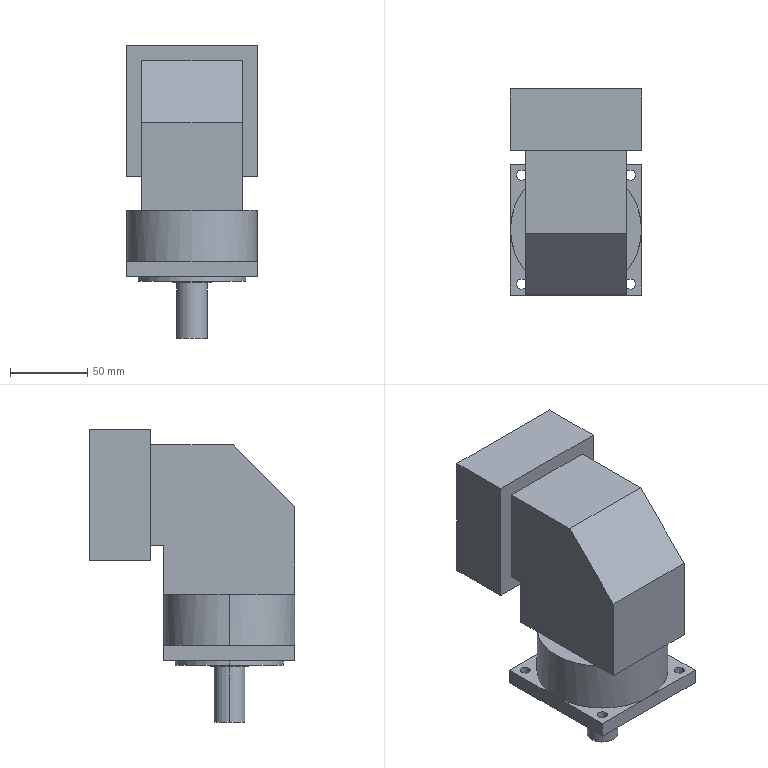Part | NX | features BREP 1 | 1 solid | 50 faces | box 85 x 133.5 x 190 mm | volume 1087253 mm3 | plane 32 | cylinder 18 | commonest cylinder face diameters 6.5 x8 20 x4 25 x2 70 x2 85 x2
STEP:
#1=CARTESIAN_POINT('',(32.5,27.386,83.2));
#2=VERTEX_POINT('',#1);
#3=CARTESIAN_POINT('',(42.5,0.,83.2));
#4=VERTEX_POINT('',#3);
#5=CARTESIAN_POINT('',(0.,0.,83.2));
#6=DIRECTION('',(0.,0.,-1.));
#7=DIRECTION('',(-1.,0.,0.));
#8=AXIS2_PLACEMENT_3D('',#5,#6,#7);
#9=CIRCLE('',#8,42.5);
#10=EDGE_CURVE('',#2,#4,#9,.T.);
#11=ORIENTED_EDGE('',*,*,#10,.T.);
#12=CARTESIAN_POINT('',(42.5,0.,50.));
#13=VERTEX_POINT('',#12);
#14=CARTESIAN_POINT('',(42.5,0.,83.2));
#15=DIRECTION('',(0.,0.,-1.));
#16=VECTOR('',#15,1000.);
#17=LINE('',#14,#16);
#18=EDGE_CURVE('',#4,#13,#17,.T.);
#19=ORIENTED_EDGE('',*,*,#18,.T.);
#20=CARTESIAN_POINT('',(0.,42.5,50.));
#21=VERTEX_POINT('',#20);
#22=CARTESIAN_POINT('',(0.,0.,50.));
#23=DIRECTION('',(0.,0.,1.));
#24=DIRECTION('',(-1.,0.,0.));
#25=AXIS2_PLACEMENT_3D('',#22,#23,#24);
#26=CIRCLE('',#25,42.5);
#27=EDGE_CURVE('',#13,#21,#26,.T.);
#28=ORIENTED_EDGE('',*,*,#27,.T.);
#29=CARTESIAN_POINT('',(-42.5,0.,50.));
#30=VERTEX_POINT('',#29);
#31=CARTESIAN_POINT('',(0.,0.,50.));
#32=DIRECTION('',(0.,0.,1.));
#33=DIRECTION('',(-1.,0.,0.));
#34=AXIS2_PLACEMENT_3D('',#31,#32,#33);
#35=CIRCLE('',#34,42.5);
#36=EDGE_CURVE('',#21,#30,#35,.T.);
#37=ORIENTED_EDGE('',*,*,#36,.T.);
#38=CARTESIAN_POINT('',(-42.5,0.,83.2));
#39=VERTEX_POINT('',#38);
#40=CARTESIAN_POINT('',(-42.5,0.,83.2));
#41=DIRECTION('',(0.,0.,-1.));
#42=VECTOR('',#41,1000.);
#43=LINE('',#40,#42);
#44=EDGE_CURVE('',#39,#30,#43,.T.);
#45=ORIENTED_EDGE('',*,*,#44,.F.);
#46=CARTESIAN_POINT('',(-32.5,27.386,83.2));
#47=VERTEX_POINT('',#46);
#48=CARTESIAN_POINT('',(0.,0.,83.2));
#49=DIRECTION('',(0.,0.,1.));
#50=DIRECTION('',(-1.,0.,0.));
#51=AXIS2_PLACEMENT_3D('',#48,#49,#50);
#52=CIRCLE('',#51,42.5);
#53=EDGE_CURVE('',#47,#39,#52,.T.);
#54=ORIENTED_EDGE('',*,*,#53,.F.);
#55=CARTESIAN_POINT('',(0.,42.5,83.2));
#56=VERTEX_POINT('',#55);
#57=CARTESIAN_POINT('',(0.,0.,83.2));
#58=DIRECTION('',(0.,0.,-1.));
#59=DIRECTION('',(-1.,0.,0.));
#60=AXIS2_PLACEMENT_3D('',#57,#58,#59);
#61=CIRCLE('',#60,42.5);
#62=EDGE_CURVE('',#47,#56,#61,.T.);
#63=ORIENTED_EDGE('',*,*,#62,.T.);
#64=CARTESIAN_POINT('',(0.,0.,83.2));
#65=DIRECTION('',(0.,0.,-1.));
#66=DIRECTION('',(-1.,0.,0.));
#67=AXIS2_PLACEMENT_3D('',#64,#65,#66);
#68=CIRCLE('',#67,42.5);
#69=EDGE_CURVE('',#56,#2,#68,.T.);
#70=ORIENTED_EDGE('',*,*,#69,.T.);
#71=EDGE_LOOP('',(#11,#19,#28,#37,#45,#54,#63,#70));
#72=FACE_BOUND('',#71,.T.);
#73=CARTESIAN_POINT('',(0.,0.,83.2));
#74=DIRECTION('',(0.,0.,-1.));
#75=DIRECTION('',(-1.,0.,0.));
#76=AXIS2_PLACEMENT_3D('',#73,#74,#75);
#77=CYLINDRICAL_SURFACE('',#76,42.5);
#78=ADVANCED_FACE('',(#72),#77,.T.);
#79=CARTESIAN_POINT('',(32.105,-35.355,50.));
#80=VERTEX_POINT('',#79);
#81=CARTESIAN_POINT('',(38.605,-35.355,50.));
#82=VERTEX_POINT('',#81);
#83=CARTESIAN_POINT('',(35.355,-35.355,50.));
#84=DIRECTION('',(0.,0.,1.));
#85=DIRECTION('',(-1.,0.,0.));
#86=AXIS2_PLACEMENT_3D('',#83,#84,#85);
#87=CIRCLE('',#86,3.25);
#88=EDGE_CURVE('',#80,#82,#87,.T.);
#89=ORIENTED_EDGE('',*,*,#88,.T.);
#90=CARTESIAN_POINT('',(38.605,-35.355,40.));
#91=VERTEX_POINT('',#90);
#92=CARTESIAN_POINT('',(38.605,-35.355,40.));
#93=DIRECTION('',(0.,0.,-1.));
#94=VECTOR('',#93,1000.);
#95=LINE('',#92,#94);
#96=EDGE_CURVE('',#82,#91,#95,.T.);
#97=ORIENTED_EDGE('',*,*,#96,.T.);
#98=CARTESIAN_POINT('',(32.105,-35.355,40.));
#99=VERTEX_POINT('',#98);
#100=CARTESIAN_POINT('',(35.355,-35.355,40.));
#101=DIRECTION('',(0.,0.,1.));
#102=DIRECTION('',(-1.,0.,0.));
#103=AXIS2_PLACEMENT_3D('',#100,#101,#102);
#104=CIRCLE('',#103,3.25);
#105=EDGE_CURVE('',#99,#91,#104,.T.);
#106=ORIENTED_EDGE('',*,*,#105,.F.);
#107=CARTESIAN_POINT('',(32.105,-35.355,40.));
#108=DIRECTION('',(0.,0.,-1.));
#109=VECTOR('',#108,1000.);
#110=LINE('',#107,#109);
#111=EDGE_CURVE('',#80,#99,#110,.T.);
#112=ORIENTED_EDGE('',*,*,#111,.F.);
#113=EDGE_LOOP('',(#89,#97,#106,#112));
#114=FACE_BOUND('',#113,.T.);
#115=CARTESIAN_POINT('',(35.355,-35.355,40.));
#116=DIRECTION('',(0.,0.,-1.));
#117=DIRECTION('',(-1.,0.,0.));
#118=AXIS2_PLACEMENT_3D('',#115,#116,#117);
#119=CYLINDRICAL_SURFACE('',#118,3.25);
#120=ADVANCED_FACE('',(#114),#119,.F.);
#121=CARTESIAN_POINT('',(-38.605,-35.355,50.));
#122=VERTEX_POINT('',#121);
#123=CARTESIAN_POINT('',(-32.105,-35.355,50.));
#124=VERTEX_POINT('',#123);
#125=CARTESIAN_POINT('',(-35.355,-35.355,50.));
#126=DIRECTION('',(0.,0.,1.));
#127=DIRECTION('',(-1.,0.,0.));
#128=AXIS2_PLACEMENT_3D('',#125,#126,#127);
#129=CIRCLE('',#128,3.25);
#130=EDGE_CURVE('',#122,#124,#129,.T.);
#131=ORIENTED_EDGE('',*,*,#130,.T.);
#132=CARTESIAN_POINT('',(-32.105,-35.355,40.));
#133=VERTEX_POINT('',#132);
#134=CARTESIAN_POINT('',(-32.105,-35.355,40.));
#135=DIRECTION('',(0.,0.,-1.));
#136=VECTOR('',#135,1000.);
#137=LINE('',#134,#136);
#138=EDGE_CURVE('',#124,#133,#137,.T.);
#139=ORIENTED_EDGE('',*,*,#138,.T.);
#140=CARTESIAN_POINT('',(-38.605,-35.355,40.));
#141=VERTEX_POINT('',#140);
#142=CARTESIAN_POINT('',(-35.355,-35.355,40.));
#143=DIRECTION('',(0.,0.,1.));
#144=DIRECTION('',(-1.,0.,0.));
#145=AXIS2_PLACEMENT_3D('',#142,#143,#144);
#146=CIRCLE('',#145,3.25);
#147=EDGE_CURVE('',#141,#133,#146,.T.);
#148=ORIENTED_EDGE('',*,*,#147,.F.);
#149=CARTESIAN_POINT('',(-38.605,-35.355,40.));
#150=DIRECTION('',(0.,0.,-1.));
#151=VECTOR('',#150,1000.);
#152=LINE('',#149,#151);
#153=EDGE_CURVE('',#122,#141,#152,.T.);
#154=ORIENTED_EDGE('',*,*,#153,.F.);
#155=EDGE_LOOP('',(#131,#139,#148,#154));
#156=FACE_BOUND('',#155,.T.);
#157=CARTESIAN_POINT('',(-35.355,-35.355,40.));
#158=DIRECTION('',(0.,0.,-1.));
#159=DIRECTION('',(-1.,0.,0.));
#160=AXIS2_PLACEMENT_3D('',#157,#158,#159);
#161=CYLINDRICAL_SURFACE('',#160,3.25);
#162=ADVANCED_FACE('',(#156),#161,.F.);
#163=CARTESIAN_POINT('',(-38.605,35.355,50.));
#164=VERTEX_POINT('',#163);
#165=CARTESIAN_POINT('',(-32.105,35.355,50.));
#166=VERTEX_POINT('',#165);
#167=CARTESIAN_POINT('',(-35.355,35.355,50.));
#168=DIRECTION('',(0.,0.,1.));
#169=DIRECTION('',(-1.,0.,0.));
#170=AXIS2_PLACEMENT_3D('',#167,#168,#169);
#171=CIRCLE('',#170,3.25);
#172=EDGE_CURVE('',#164,#166,#171,.T.);
#173=ORIENTED_EDGE('',*,*,#172,.T.);
#174=CARTESIAN_POINT('',(-32.105,35.355,40.));
#175=VERTEX_POINT('',#174);
#176=CARTESIAN_POINT('',(-32.105,35.355,40.));
#177=DIRECTION('',(0.,0.,-1.));
#178=VECTOR('',#177,1000.);
#179=LINE('',#176,#178);
#180=EDGE_CURVE('',#166,#175,#179,.T.);
#181=ORIENTED_EDGE('',*,*,#180,.T.);
#182=CARTESIAN_POINT('',(-38.605,35.355,40.));
#183=VERTEX_POINT('',#182);
#184=CARTESIAN_POINT('',(-35.355,35.355,40.));
#185=DIRECTION('',(0.,0.,1.));
#186=DIRECTION('',(-1.,0.,0.));
#187=AXIS2_PLACEMENT_3D('',#184,#185,#186);
#188=CIRCLE('',#187,3.25);
#189=EDGE_CURVE('',#183,#175,#188,.T.);
#190=ORIENTED_EDGE('',*,*,#189,.F.);
#191=CARTESIAN_POINT('',(-38.605,35.355,40.));
#192=DIRECTION('',(0.,0.,-1.));
#193=VECTOR('',#192,1000.);
#194=LINE('',#191,#193);
#195=EDGE_CURVE('',#164,#183,#194,.T.);
#196=ORIENTED_EDGE('',*,*,#195,.F.);
#197=EDGE_LOOP('',(#173,#181,#190,#196));
#198=FACE_BOUND('',#197,.T.);
#199=CARTESIAN_POINT('',(-35.355,35.355,40.));
#200=DIRECTION('',(0.,0.,-1.));
#201=DIRECTION('',(-1.,0.,0.));
#202=AXIS2_PLACEMENT_3D('',#199,#200,#201);
#203=CYLINDRICAL_SURFACE('',#202,3.25);
#204=ADVANCED_FACE('',(#198),#203,.F.);
#205=CARTESIAN_POINT('',(32.105,35.355,50.));
#206=VERTEX_POINT('',#205);
#207=CARTESIAN_POINT('',(38.605,35.355,50.));
#208=VERTEX_POINT('',#207);
#209=CARTESIAN_POINT('',(35.355,35.355,50.));
#210=DIRECTION('',(0.,0.,1.));
#211=DIRECTION('',(-1.,0.,0.));
#212=AXIS2_PLACEMENT_3D('',#209,#210,#211);
#213=CIRCLE('',#212,3.25);
#214=EDGE_CURVE('',#206,#208,#213,.T.);
#215=ORIENTED_EDGE('',*,*,#214,.T.);
#216=CARTESIAN_POINT('',(38.605,35.355,40.));
#217=VERTEX_POINT('',#216);
#218=CARTESIAN_POINT('',(38.605,35.355,40.));
#219=DIRECTION('',(0.,0.,-1.));
#220=VECTOR('',#219,1000.);
#221=LINE('',#218,#220);
#222=EDGE_CURVE('',#208,#217,#221,.T.);
#223=ORIENTED_EDGE('',*,*,#222,.T.);
#224=CARTESIAN_POINT('',(32.105,35.355,40.));
#225=VERTEX_POINT('',#224);
#226=CARTESIAN_POINT('',(35.355,35.355,40.));
#227=DIRECTION('',(0.,0.,1.));
#228=DIRECTION('',(-1.,0.,0.));
#229=AXIS2_PLACEMENT_3D('',#226,#227,#228);
#230=CIRCLE('',#229,3.25);
#231=EDGE_CURVE('',#225,#217,#230,.T.);
#232=ORIENTED_EDGE('',*,*,#231,.F.);
#233=CARTESIAN_POINT('',(32.105,35.355,40.));
#234=DIRECTION('',(0.,0.,-1.));
#235=VECTOR('',#234,1000.);
#236=LINE('',#233,#235);
#237=EDGE_CURVE('',#206,#225,#236,.T.);
#238=ORIENTED_EDGE('',*,*,#237,.F.);
#239=EDGE_LOOP('',(#215,#223,#232,#238));
#240=FACE_BOUND('',#239,.T.);
#241=CARTESIAN_POINT('',(35.355,35.355,40.));
#242=DIRECTION('',(0.,0.,-1.));
#243=DIRECTION('',(-1.,0.,0.));
#244=AXIS2_PLACEMENT_3D('',#241,#242,#243);
#245=CYLINDRICAL_SURFACE('',#244,3.25);
#246=ADVANCED_FACE('',(#240),#245,.F.);
#247=CARTESIAN_POINT('',(0.,81.,137.5));
#248=VERTEX_POINT('',#247);
#249=CARTESIAN_POINT('',(0.,81.,157.5));
#250=VERTEX_POINT('',#249);
#251=CARTESIAN_POINT('',(0.,81.,147.5));
#252=DIRECTION('',(0.,1.,0.));
#253=DIRECTION('',(0.,0.,1.));
#254=AXIS2_PLACEMENT_3D('',#251,#252,#253);
#255=CIRCLE('',#254,10.);
#256=EDGE_CURVE('',#248,#250,#255,.T.);
#257=ORIENTED_EDGE('',*,*,#256,.F.);
#258=CARTESIAN_POINT('',(0.,91.,137.5));
#259=VERTEX_POINT('',#258);
#260=CARTESIAN_POINT('',(0.,81.,137.5));
#261=DIRECTION('',(0.,1.,0.));
#262=VECTOR('',#261,1000.);
#263=LINE('',#260,#262);
#264=EDGE_CURVE('',#259,#248,#263,.F.);
#265=ORIENTED_EDGE('',*,*,#264,.F.);
#266=CARTESIAN_POINT('',(0.,91.,157.5));
#267=VERTEX_POINT('',#266);
#268=CARTESIAN_POINT('',(0.,91.,147.5));
#269=DIRECTION('',(0.,1.,0.));
#270=DIRECTION('',(0.,0.,1.));
#271=AXIS2_PLACEMENT_3D('',#268,#269,#270);
#272=CIRCLE('',#271,10.);
#273=EDGE_CURVE('',#259,#267,#272,.T.);
#274=ORIENTED_EDGE('',*,*,#273,.T.);
#275=CARTESIAN_POINT('',(0.,81.,157.5));
#276=DIRECTION('',(0.,1.,0.));
#277=VECTOR('',#276,1000.);
#278=LINE('',#275,#277);
#279=EDGE_CURVE('',#267,#250,#278,.F.);
#280=ORIENTED_EDGE('',*,*,#279,.T.);
#281=EDGE_LOOP('',(#257,#265,#274,#280));
#282=FACE_BOUND('',#281,.T.);
#283=CARTESIAN_POINT('',(0.,81.,147.5));
#284=DIRECTION('',(0.,1.,0.));
#285=DIRECTION('',(0.,0.,1.));
#286=AXIS2_PLACEMENT_3D('',#283,#284,#285);
#287=CYLINDRICAL_SURFACE('',#286,10.);
#288=ADVANCED_FACE('',(#282),#287,.F.);
#289=CARTESIAN_POINT('',(-35.,0.,40.));
#290=VERTEX_POINT('',#289);
#291=CARTESIAN_POINT('',(35.,0.,40.));
#292=VERTEX_POINT('',#291);
#293=CARTESIAN_POINT('',(0.,0.,40.));
#294=DIRECTION('',(0.,0.,-1.));
#295=DIRECTION('',(-1.,0.,0.));
#296=AXIS2_PLACEMENT_3D('',#293,#294,#295);
#297=CIRCLE('',#296,35.);
#298=EDGE_CURVE('',#290,#292,#297,.T.);
#299=ORIENTED_EDGE('',*,*,#298,.T.);
#300=CARTESIAN_POINT('',(35.,0.,37.));
#301=VERTEX_POINT('',#300);
#302=CARTESIAN_POINT('',(35.,0.,40.));
#303=DIRECTION('',(0.,0.,-1.));
#304=VECTOR('',#303,1000.);
#305=LINE('',#302,#304);
#306=EDGE_CURVE('',#292,#301,#305,.T.);
#307=ORIENTED_EDGE('',*,*,#306,.T.);
#308=CARTESIAN_POINT('',(-35.,0.,37.));
#309=VERTEX_POINT('',#308);
#310=CARTESIAN_POINT('',(0.,0.,37.));
#311=DIRECTION('',(0.,0.,1.));
#312=DIRECTION('',(-1.,0.,0.));
#313=AXIS2_PLACEMENT_3D('',#310,#311,#312);
#314=CIRCLE('',#313,35.);
#315=EDGE_CURVE('',#301,#309,#314,.T.);
#316=ORIENTED_EDGE('',*,*,#315,.T.);
#317=CARTESIAN_POINT('',(-35.,0.,40.));
#318=DIRECTION('',(0.,0.,-1.));
#319=VECTOR('',#318,1000.);
#320=LINE('',#317,#319);
#321=EDGE_CURVE('',#290,#309,#320,.T.);
#322=ORIENTED_EDGE('',*,*,#321,.F.);
#323=EDGE_LOOP('',(#299,#307,#316,#322));
#324=FACE_BOUND('',#323,.T.);
#325=CARTESIAN_POINT('',(0.,0.,40.));
#326=DIRECTION('',(0.,0.,-1.));
#327=DIRECTION('',(-1.,0.,0.));
#328=AXIS2_PLACEMENT_3D('',#325,#326,#327);
#329=CYLINDRICAL_SURFACE('',#328,35.);
#330=ADVANCED_FACE('',(#324),#329,.T.);
#331=CARTESIAN_POINT('',(-12.5,0.,37.));
#332=VERTEX_POINT('',#331);
#333=CARTESIAN_POINT('',(12.5,0.,37.));
#334=VERTEX_POINT('',#333);
#335=CARTESIAN_POINT('',(0.,0.,37.));
#336=DIRECTION('',(0.,0.,-1.));
#337=DIRECTION('',(-1.,0.,0.));
#338=AXIS2_PLACEMENT_3D('',#335,#336,#337);
#339=CIRCLE('',#338,12.5);
#340=EDGE_CURVE('',#332,#334,#339,.T.);
#341=ORIENTED_EDGE('',*,*,#340,.T.);
#342=CARTESIAN_POINT('',(12.5,0.,36.));
#343=VERTEX_POINT('',#342);
#344=CARTESIAN_POINT('',(12.5,0.,37.));
#345=DIRECTION('',(0.,0.,-1.));
#346=VECTOR('',#345,1000.);
#347=LINE('',#344,#346);
#348=EDGE_CURVE('',#334,#343,#347,.T.);
#349=ORIENTED_EDGE('',*,*,#348,.T.);
#350=CARTESIAN_POINT('',(-12.5,0.,36.));
#351=VERTEX_POINT('',#350);
#352=CARTESIAN_POINT('',(0.,0.,36.));
#353=DIRECTION('',(0.,0.,1.));
#354=DIRECTION('',(-1.,0.,0.));
#355=AXIS2_PLACEMENT_3D('',#352,#353,#354);
#356=CIRCLE('',#355,12.5);
#357=EDGE_CURVE('',#343,#351,#356,.T.);
#358=ORIENTED_EDGE('',*,*,#357,.T.);
#359=CARTESIAN_POINT('',(-12.5,0.,37.));
#360=DIRECTION('',(0.,0.,-1.));
#361=VECTOR('',#360,1000.);
#362=LINE('',#359,#361);
#363=EDGE_CURVE('',#332,#351,#362,.T.);
#364=ORIENTED_EDGE('',*,*,#363,.F.);
#365=EDGE_LOOP('',(#341,#349,#358,#364));
#366=FACE_BOUND('',#365,.T.);
#367=CARTESIAN_POINT('',(0.,0.,37.));
#368=DIRECTION('',(0.,0.,-1.));
#369=DIRECTION('',(-1.,0.,0.));
#370=AXIS2_PLACEMENT_3D('',#367,#368,#369);
#371=CYLINDRICAL_SURFACE('',#370,12.5);
#372=ADVANCED_FACE('',(#366),#371,.T.);
#373=CARTESIAN_POINT('',(-10.,0.,36.));
#374=VERTEX_POINT('',#373);
#375=CARTESIAN_POINT('',(10.,0.,36.));
#376=VERTEX_POINT('',#375);
#377=CARTESIAN_POINT('',(0.,0.,36.));
#378=DIRECTION('',(0.,0.,-1.));
#379=DIRECTION('',(-1.,0.,0.));
#380=AXIS2_PLACEMENT_3D('',#377,#378,#379);
#381=CIRCLE('',#380,10.);
#382=EDGE_CURVE('',#374,#376,#381,.T.);
#383=ORIENTED_EDGE('',*,*,#382,.T.);
#384=CARTESIAN_POINT('',(10.,0.,0.));
#385=VERTEX_POINT('',#384);
#386=CARTESIAN_POINT('',(10.,0.,36.));
#387=DIRECTION('',(0.,0.,-1.));
#388=VECTOR('',#387,1000.);
#389=LINE('',#386,#388);
#390=EDGE_CURVE('',#376,#385,#389,.T.);
#391=ORIENTED_EDGE('',*,*,#390,.T.);
#392=CARTESIAN_POINT('',(-10.,0.,0.));
#393=VERTEX_POINT('',#392);
#394=CARTESIAN_POINT('',(0.,0.,0.));
#395=DIRECTION('',(0.,0.,1.));
#396=DIRECTION('',(-1.,0.,0.));
#397=AXIS2_PLACEMENT_3D('',#394,#395,#396);
#398=CIRCLE('',#397,10.);
#399=EDGE_CURVE('',#385,#393,#398,.T.);
#400=ORIENTED_EDGE('',*,*,#399,.T.);
#401=CARTESIAN_POINT('',(-10.,0.,36.));
#402=DIRECTION('',(0.,0.,-1.));
#403=VECTOR('',#402,1000.);
#404=LINE('',#401,#403);
#405=EDGE_CURVE('',#374,#393,#404,.T.);
#406=ORIENTED_EDGE('',*,*,#405,.F.);
#407=EDGE_LOOP('',(#383,#391,#400,#406));
#408=FACE_BOUND('',#407,.T.);
#409=CARTESIAN_POINT('',(0.,0.,36.));
#410=DIRECTION('',(0.,0.,-1.));
#411=DIRECTION('',(-1.,0.,0.));
#412=AXIS2_PLACEMENT_3D('',#409,#410,#411);
#413=CYLINDRICAL_SURFACE('',#412,10.);
#414=ADVANCED_FACE('',(#408),#413,.T.);
#415=CARTESIAN_POINT('',(-32.5,-42.5,83.2));
#416=VERTEX_POINT('',#415);
#417=CARTESIAN_POINT('',(-32.5,-42.5,140.));
#418=VERTEX_POINT('',#417);
#419=CARTESIAN_POINT('',(-32.5,-42.5,180.));
#420=DIRECTION('',(0.,0.,1.));
#421=VECTOR('',#420,1000.);
#422=LINE('',#419,#421);
#423=EDGE_CURVE('',#416,#418,#422,.T.);
#424=ORIENTED_EDGE('',*,*,#423,.T.);
#425=CARTESIAN_POINT('',(-32.5,-2.5,180.));
#426=VERTEX_POINT('',#425);
#427=CARTESIAN_POINT('',(-32.5,-42.5,140.));
#428=DIRECTION('',(0.,0.7071,0.7071));
#429=VECTOR('',#428,1000.);
#430=LINE('',#427,#429);
#431=EDGE_CURVE('',#418,#426,#430,.T.);
#432=ORIENTED_EDGE('',*,*,#431,.T.);
#433=CARTESIAN_POINT('',(-32.5,51.,180.));
#434=VERTEX_POINT('',#433);
#435=CARTESIAN_POINT('',(-32.5,-42.5,180.));
#436=DIRECTION('',(0.,1.,0.));
#437=VECTOR('',#436,1000.);
#438=LINE('',#435,#437);
#439=EDGE_CURVE('',#426,#434,#438,.T.);
#440=ORIENTED_EDGE('',*,*,#439,.T.);
#441=CARTESIAN_POINT('',(-32.5,51.,115.));
#442=VERTEX_POINT('',#441);
#443=CARTESIAN_POINT('',(-32.5,51.,180.));
#444=DIRECTION('',(0.,0.,-1.));
#445=VECTOR('',#444,1000.);
#446=LINE('',#443,#445);
#447=EDGE_CURVE('',#434,#442,#446,.T.);
#448=ORIENTED_EDGE('',*,*,#447,.T.);
#449=CARTESIAN_POINT('',(-32.5,42.5,115.));
#450=VERTEX_POINT('',#449);
#451=CARTESIAN_POINT('',(-32.5,-42.5,115.));
#452=DIRECTION('',(0.,-1.,0.));
#453=VECTOR('',#452,1000.);
#454=LINE('',#451,#453);
#455=EDGE_CURVE('',#442,#450,#454,.T.);
#456=ORIENTED_EDGE('',*,*,#455,.T.);
#457=CARTESIAN_POINT('',(-32.5,42.5,83.2));
#458=VERTEX_POINT('',#457);
#459=CARTESIAN_POINT('',(-32.5,42.5,180.));
#460=DIRECTION('',(0.,0.,-1.));
#461=VECTOR('',#460,1000.);
#462=LINE('',#459,#461);
#463=EDGE_CURVE('',#450,#458,#462,.T.);
#464=ORIENTED_EDGE('',*,*,#463,.T.);
#465=CARTESIAN_POINT('',(-32.5,-42.5,83.2));
#466=DIRECTION('',(0.,-1.,0.));
#467=VECTOR('',#466,1000.);
#468=LINE('',#465,#467);
#469=EDGE_CURVE('',#458,#47,#468,.T.);
#470=ORIENTED_EDGE('',*,*,#469,.T.);
#471=CARTESIAN_POINT('',(-32.5,-27.386,83.2));
#472=VERTEX_POINT('',#471);
#473=CARTESIAN_POINT('',(-32.5,-42.5,83.2));
#474=DIRECTION('',(0.,-1.,0.));
#475=VECTOR('',#474,1000.);
#476=LINE('',#473,#475);
#477=EDGE_CURVE('',#47,#472,#476,.T.);
#478=ORIENTED_EDGE('',*,*,#477,.T.);
#479=CARTESIAN_POINT('',(-32.5,-42.5,83.2));
#480=DIRECTION('',(0.,-1.,0.));
#481=VECTOR('',#480,1000.);
#482=LINE('',#479,#481);
#483=EDGE_CURVE('',#472,#416,#482,.T.);
#484=ORIENTED_EDGE('',*,*,#483,.T.);
#485=EDGE_LOOP('',(#424,#432,#440,#448,#456,#464,#470,#478,#484));
#486=FACE_BOUND('',#485,.T.);
#487=CARTESIAN_POINT('',(-32.5,-42.5,180.));
#488=DIRECTION('',(-1.,0.,0.));
#489=DIRECTION('',(0.,0.,1.));
#490=AXIS2_PLACEMENT_3D('',#487,#488,#489);
#491=PLANE('',#490);
#492=ADVANCED_FACE('',(#486),#491,.T.);
#493=CARTESIAN_POINT('',(32.5,-42.5,140.));
#494=VERTEX_POINT('',#493);
#495=CARTESIAN_POINT('',(32.5,-42.5,140.));
#496=DIRECTION('',(-1.,0.,0.));
#497=VECTOR('',#496,1000.);
#498=LINE('',#495,#497);
#499=EDGE_CURVE('',#494,#418,#498,.T.);
#500=ORIENTED_EDGE('',*,*,#499,.F.);
#501=CARTESIAN_POINT('',(32.5,-2.5,180.));
#502=VERTEX_POINT('',#501);
#503=CARTESIAN_POINT('',(32.5,-2.5,180.));
#504=DIRECTION('',(0.,-0.7071,-0.7071));
#505=VECTOR('',#504,1000.);
#506=LINE('',#503,#505);
#507=EDGE_CURVE('',#502,#494,#506,.T.);
#508=ORIENTED_EDGE('',*,*,#507,.F.);
#509=CARTESIAN_POINT('',(32.5,-2.5,180.));
#510=DIRECTION('',(1.,0.,0.));
#511=VECTOR('',#510,1000.);
#512=LINE('',#509,#511);
#513=EDGE_CURVE('',#426,#502,#512,.T.);
#514=ORIENTED_EDGE('',*,*,#513,.F.);
#515=ORIENTED_EDGE('',*,*,#431,.F.);
#516=EDGE_LOOP('',(#500,#508,#514,#515));
#517=FACE_BOUND('',#516,.T.);
#518=CARTESIAN_POINT('',(32.5,-2.5,180.));
#519=DIRECTION('',(0.,0.7071,-0.7071));
#520=DIRECTION('',(-1.,0.,0.));
#521=AXIS2_PLACEMENT_3D('',#518,#519,#520);
#522=PLANE('',#521);
#523=ADVANCED_FACE('',(#517),#522,.F.);
#524=CARTESIAN_POINT('',(0.,-42.5,83.2));
#525=VERTEX_POINT('',#524);
#526=CARTESIAN_POINT('',(32.5,-42.5,83.2));
#527=DIRECTION('',(-1.,0.,0.));
#528=VECTOR('',#527,1000.);
#529=LINE('',#526,#528);
#530=EDGE_CURVE('',#525,#416,#529,.T.);
#531=ORIENTED_EDGE('',*,*,#530,.F.);
#532=CARTESIAN_POINT('',(32.5,-42.5,83.2));
#533=VERTEX_POINT('',#532);
#534=CARTESIAN_POINT('',(32.5,-42.5,83.2));
#535=DIRECTION('',(-1.,0.,0.));
#536=VECTOR('',#535,1000.);
#537=LINE('',#534,#536);
#538=EDGE_CURVE('',#533,#525,#537,.T.);
#539=ORIENTED_EDGE('',*,*,#538,.F.);
#540=CARTESIAN_POINT('',(32.5,-42.5,83.2));
#541=DIRECTION('',(0.,0.,-1.));
#542=VECTOR('',#541,1000.);
#543=LINE('',#540,#542);
#544=EDGE_CURVE('',#494,#533,#543,.T.);
#545=ORIENTED_EDGE('',*,*,#544,.F.);
#546=ORIENTED_EDGE('',*,*,#499,.T.);
#547=ORIENTED_EDGE('',*,*,#423,.F.);
#548=EDGE_LOOP('',(#531,#539,#545,#546,#547));
#549=FACE_BOUND('',#548,.T.);
#550=CARTESIAN_POINT('',(32.5,-42.5,83.2));
#551=DIRECTION('',(0.,1.,0.));
#552=DIRECTION('',(0.,0.,-1.));
#553=AXIS2_PLACEMENT_3D('',#550,#551,#552);
#554=PLANE('',#553);
#555=ADVANCED_FACE('',(#549),#554,.F.);
#556=CARTESIAN_POINT('',(0.,0.,83.2));
#557=DIRECTION('',(0.,0.,-1.));
#558=DIRECTION('',(-1.,0.,0.));
#559=AXIS2_PLACEMENT_3D('',#556,#557,#558);
#560=CIRCLE('',#559,42.5);
#561=EDGE_CURVE('',#525,#472,#560,.T.);
#562=ORIENTED_EDGE('',*,*,#561,.F.);
#563=ORIENTED_EDGE('',*,*,#530,.T.);
#564=ORIENTED_EDGE('',*,*,#483,.F.);
#565=EDGE_LOOP('',(#562,#563,#564));
#566=FACE_BOUND('',#565,.T.);
#567=CARTESIAN_POINT('',(32.5,42.5,83.2));
#568=DIRECTION('',(0.,0.,1.));
#569=DIRECTION('',(1.,0.,0.));
#570=AXIS2_PLACEMENT_3D('',#567,#568,#569);
#571=PLANE('',#570);
#572=ADVANCED_FACE('',(#566),#571,.F.);
#573=ORIENTED_EDGE('',*,*,#53,.T.);
#574=CARTESIAN_POINT('',(0.,0.,83.2));
#575=DIRECTION('',(0.,0.,1.));
#576=DIRECTION('',(-1.,0.,0.));
#577=AXIS2_PLACEMENT_3D('',#574,#575,#576);
#578=CIRCLE('',#577,42.5);
#579=EDGE_CURVE('',#39,#472,#578,.T.);
#580=ORIENTED_EDGE('',*,*,#579,.T.);
#581=ORIENTED_EDGE('',*,*,#477,.F.);
#582=EDGE_LOOP('',(#573,#580,#581));
#583=FACE_BOUND('',#582,.T.);
#584=CARTESIAN_POINT('',(-42.5,42.5,83.2));
#585=DIRECTION('',(0.,0.,1.));
#586=DIRECTION('',(1.,0.,0.));
#587=AXIS2_PLACEMENT_3D('',#584,#585,#586);
#588=PLANE('',#587);
#589=ADVANCED_FACE('',(#583),#588,.T.);
#590=ORIENTED_EDGE('',*,*,#62,.F.);
#591=ORIENTED_EDGE('',*,*,#469,.F.);
#592=CARTESIAN_POINT('',(32.5,42.5,83.2));
#593=DIRECTION('',(-1.,0.,0.));
#594=VECTOR('',#593,1000.);
#595=LINE('',#592,#594);
#596=EDGE_CURVE('',#56,#458,#595,.T.);
#597=ORIENTED_EDGE('',*,*,#596,.F.);
#598=EDGE_LOOP('',(#590,#591,#597));
#599=FACE_BOUND('',#598,.T.);
#600=CARTESIAN_POINT('',(32.5,42.5,83.2));
#601=DIRECTION('',(0.,0.,1.));
#602=DIRECTION('',(1.,0.,0.));
#603=AXIS2_PLACEMENT_3D('',#600,#601,#602);
#604=PLANE('',#603);
#605=ADVANCED_FACE('',(#599),#604,.F.);
#606=CARTESIAN_POINT('',(32.5,42.5,115.));
#607=VERTEX_POINT('',#606);
#608=CARTESIAN_POINT('',(32.5,42.5,115.));
#609=DIRECTION('',(-1.,0.,0.));
#610=VECTOR('',#609,1000.);
#611=LINE('',#608,#610);
#612=EDGE_CURVE('',#607,#450,#611,.T.);
#613=ORIENTED_EDGE('',*,*,#612,.F.);
#614=CARTESIAN_POINT('',(32.5,42.5,83.2));
#615=VERTEX_POINT('',#614);
#616=CARTESIAN_POINT('',(32.5,42.5,83.2));
#617=DIRECTION('',(0.,0.,1.));
#618=VECTOR('',#617,1000.);
#619=LINE('',#616,#618);
#620=EDGE_CURVE('',#615,#607,#619,.T.);
#621=ORIENTED_EDGE('',*,*,#620,.F.);
#622=CARTESIAN_POINT('',(32.5,42.5,83.2));
#623=DIRECTION('',(1.,0.,0.));
#624=VECTOR('',#623,1000.);
#625=LINE('',#622,#624);
#626=EDGE_CURVE('',#56,#615,#625,.T.);
#627=ORIENTED_EDGE('',*,*,#626,.F.);
#628=ORIENTED_EDGE('',*,*,#596,.T.);
#629=ORIENTED_EDGE('',*,*,#463,.F.);
#630=EDGE_LOOP('',(#613,#621,#627,#628,#629));
#631=FACE_BOUND('',#630,.T.);
#632=CARTESIAN_POINT('',(32.5,42.5,83.2));
#633=DIRECTION('',(0.,-1.,0.));
#634=DIRECTION('',(0.,0.,-1.));
#635=AXIS2_PLACEMENT_3D('',#632,#633,#634);
#636=PLANE('',#635);
#637=ADVANCED_FACE('',(#631),#636,.F.);
#638=CARTESIAN_POINT('',(32.5,51.,115.));
#639=VERTEX_POINT('',#638);
#640=CARTESIAN_POINT('',(32.5,51.,115.));
#641=DIRECTION('',(-1.,0.,0.));
#642=VECTOR('',#641,1000.);
#643=LINE('',#640,#642);
#644=EDGE_CURVE('',#639,#442,#643,.T.);
#645=ORIENTED_EDGE('',*,*,#644,.F.);
#646=CARTESIAN_POINT('',(32.5,42.5,115.));
#647=DIRECTION('',(0.,1.,0.));
#648=VECTOR('',#647,1000.);
#649=LINE('',#646,#648);
#650=EDGE_CURVE('',#607,#639,#649,.T.);
#651=ORIENTED_EDGE('',*,*,#650,.F.);
#652=ORIENTED_EDGE('',*,*,#612,.T.);
#653=ORIENTED_EDGE('',*,*,#455,.F.);
#654=EDGE_LOOP('',(#645,#651,#652,#653));
#655=FACE_BOUND('',#654,.T.);
#656=CARTESIAN_POINT('',(32.5,42.5,115.));
#657=DIRECTION('',(0.,0.,1.));
#658=DIRECTION('',(1.,0.,0.));
#659=AXIS2_PLACEMENT_3D('',#656,#657,#658);
#660=PLANE('',#659);
#661=ADVANCED_FACE('',(#655),#660,.F.);
#662=CARTESIAN_POINT('',(42.5,51.,105.));
#663=VERTEX_POINT('',#662);
#664=CARTESIAN_POINT('',(-42.5,51.,105.));
#665=VERTEX_POINT('',#664);
#666=CARTESIAN_POINT('',(42.5,51.,105.));
#667=DIRECTION('',(-1.,0.,0.));
#668=VECTOR('',#667,1000.);
#669=LINE('',#666,#668);
#670=EDGE_CURVE('',#663,#665,#669,.T.);
#671=ORIENTED_EDGE('',*,*,#670,.F.);
#672=CARTESIAN_POINT('',(42.5,51.,190.));
#673=VERTEX_POINT('',#672);
#674=CARTESIAN_POINT('',(42.5,51.,190.));
#675=DIRECTION('',(0.,0.,-1.));
#676=VECTOR('',#675,1000.);
#677=LINE('',#674,#676);
#678=EDGE_CURVE('',#673,#663,#677,.T.);
#679=ORIENTED_EDGE('',*,*,#678,.F.);
#680=CARTESIAN_POINT('',(-42.5,51.,190.));
#681=VERTEX_POINT('',#680);
#682=CARTESIAN_POINT('',(42.5,51.,190.));
#683=DIRECTION('',(1.,0.,0.));
#684=VECTOR('',#683,1000.);
#685=LINE('',#682,#684);
#686=EDGE_CURVE('',#681,#673,#685,.T.);
#687=ORIENTED_EDGE('',*,*,#686,.F.);
#688=CARTESIAN_POINT('',(-42.5,51.,190.));
#689=DIRECTION('',(0.,0.,1.));
#690=VECTOR('',#689,1000.);
#691=LINE('',#688,#690);
#692=EDGE_CURVE('',#665,#681,#691,.T.);
#693=ORIENTED_EDGE('',*,*,#692,.F.);
#694=EDGE_LOOP('',(#671,#679,#687,#693));
#695=FACE_BOUND('',#694,.T.);
#696=CARTESIAN_POINT('',(32.5,51.,180.));
#697=VERTEX_POINT('',#696);
#698=CARTESIAN_POINT('',(32.5,51.,190.));
#699=DIRECTION('',(0.,0.,1.));
#700=VECTOR('',#699,1000.);
#701=LINE('',#698,#700);
#702=EDGE_CURVE('',#639,#697,#701,.T.);
#703=ORIENTED_EDGE('',*,*,#702,.F.);
#704=ORIENTED_EDGE('',*,*,#644,.T.);
#705=ORIENTED_EDGE('',*,*,#447,.F.);
#706=CARTESIAN_POINT('',(42.5,51.,180.));
#707=DIRECTION('',(-1.,0.,0.));
#708=VECTOR('',#707,1000.);
#709=LINE('',#706,#708);
#710=EDGE_CURVE('',#697,#434,#709,.T.);
#711=ORIENTED_EDGE('',*,*,#710,.F.);
#712=EDGE_LOOP('',(#703,#704,#705,#711));
#713=FACE_BOUND('',#712,.T.);
#714=CARTESIAN_POINT('',(42.5,51.,190.));
#715=DIRECTION('',(0.,1.,0.));
#716=DIRECTION('',(1.,0.,0.));
#717=AXIS2_PLACEMENT_3D('',#714,#715,#716);
#718=PLANE('',#717);
#719=ADVANCED_FACE('',(#695,#713),#718,.F.);
#720=ORIENTED_EDGE('',*,*,#513,.T.);
#721=CARTESIAN_POINT('',(32.5,51.,180.));
#722=DIRECTION('',(0.,-1.,0.));
#723=VECTOR('',#722,1000.);
#724=LINE('',#721,#723);
#725=EDGE_CURVE('',#697,#502,#724,.T.);
#726=ORIENTED_EDGE('',*,*,#725,.F.);
#727=ORIENTED_EDGE('',*,*,#710,.T.);
#728=ORIENTED_EDGE('',*,*,#439,.F.);
#729=EDGE_LOOP('',(#720,#726,#727,#728));
#730=FACE_BOUND('',#729,.T.);
#731=CARTESIAN_POINT('',(32.5,51.,180.));
#732=DIRECTION('',(0.,0.,-1.));
#733=DIRECTION('',(0.,-1.,0.));
#734=AXIS2_PLACEMENT_3D('',#731,#732,#733);
#735=PLANE('',#734);
#736=ADVANCED_FACE('',(#730),#735,.F.);
#737=ORIENTED_EDGE('',*,*,#507,.T.);
#738=ORIENTED_EDGE('',*,*,#544,.T.);
#739=CARTESIAN_POINT('',(32.5,-27.386,83.2));
#740=VERTEX_POINT('',#739);
#741=CARTESIAN_POINT('',(32.5,-42.5,83.2));
#742=DIRECTION('',(0.,-1.,0.));
#743=VECTOR('',#742,1000.);
#744=LINE('',#741,#743);
#745=EDGE_CURVE('',#740,#533,#744,.T.);
#746=ORIENTED_EDGE('',*,*,#745,.F.);
#747=CARTESIAN_POINT('',(32.5,-42.5,83.2));
#748=DIRECTION('',(0.,-1.,0.));
#749=VECTOR('',#748,1000.);
#750=LINE('',#747,#749);
#751=EDGE_CURVE('',#2,#740,#750,.T.);
#752=ORIENTED_EDGE('',*,*,#751,.F.);
#753=CARTESIAN_POINT('',(32.5,-42.5,83.2));
#754=DIRECTION('',(0.,-1.,0.));
#755=VECTOR('',#754,1000.);
#756=LINE('',#753,#755);
#757=EDGE_CURVE('',#615,#2,#756,.T.);
#758=ORIENTED_EDGE('',*,*,#757,.F.);
#759=ORIENTED_EDGE('',*,*,#620,.T.);
#760=ORIENTED_EDGE('',*,*,#650,.T.);
#761=ORIENTED_EDGE('',*,*,#702,.T.);
#762=ORIENTED_EDGE('',*,*,#725,.T.);
#763=EDGE_LOOP('',(#737,#738,#746,#752,#758,#759,#760,#761,#762));
#764=FACE_BOUND('',#763,.T.);
#765=CARTESIAN_POINT('',(32.5,-42.5,180.));
#766=DIRECTION('',(-1.,0.,0.));
#767=DIRECTION('',(0.,0.,1.));
#768=AXIS2_PLACEMENT_3D('',#765,#766,#767);
#769=PLANE('',#768);
#770=ADVANCED_FACE('',(#764),#769,.F.);
#771=CARTESIAN_POINT('',(0.,0.,83.2));
#772=DIRECTION('',(0.,0.,-1.));
#773=DIRECTION('',(-1.,0.,0.));
#774=AXIS2_PLACEMENT_3D('',#771,#772,#773);
#775=CIRCLE('',#774,42.5);
#776=EDGE_CURVE('',#740,#525,#775,.T.);
#777=ORIENTED_EDGE('',*,*,#776,.F.);
#778=ORIENTED_EDGE('',*,*,#745,.T.);
#779=ORIENTED_EDGE('',*,*,#538,.T.);
#780=EDGE_LOOP('',(#777,#778,#779));
#781=FACE_BOUND('',#780,.T.);
#782=CARTESIAN_POINT('',(32.5,42.5,83.2));
#783=DIRECTION('',(0.,0.,1.));
#784=DIRECTION('',(1.,0.,0.));
#785=AXIS2_PLACEMENT_3D('',#782,#783,#784);
#786=PLANE('',#785);
#787=ADVANCED_FACE('',(#781),#786,.F.);
#788=ORIENTED_EDGE('',*,*,#18,.F.);
#789=CARTESIAN_POINT('',(0.,0.,83.2));
#790=DIRECTION('',(0.,0.,-1.));
#791=DIRECTION('',(-1.,0.,0.));
#792=AXIS2_PLACEMENT_3D('',#789,#790,#791);
#793=CIRCLE('',#792,42.5);
#794=EDGE_CURVE('',#4,#740,#793,.T.);
#795=ORIENTED_EDGE('',*,*,#794,.T.);
#796=ORIENTED_EDGE('',*,*,#776,.T.);
#797=ORIENTED_EDGE('',*,*,#561,.T.);
#798=ORIENTED_EDGE('',*,*,#579,.F.);
#799=ORIENTED_EDGE('',*,*,#44,.T.);
#800=CARTESIAN_POINT('',(0.,-42.5,50.));
#801=VERTEX_POINT('',#800);
#802=CARTESIAN_POINT('',(0.,0.,50.));
#803=DIRECTION('',(0.,0.,1.));
#804=DIRECTION('',(-1.,0.,0.));
#805=AXIS2_PLACEMENT_3D('',#802,#803,#804);
#806=CIRCLE('',#805,42.5);
#807=EDGE_CURVE('',#30,#801,#806,.T.);
#808=ORIENTED_EDGE('',*,*,#807,.T.);
#809=CARTESIAN_POINT('',(0.,0.,50.));
#810=DIRECTION('',(0.,0.,1.));
#811=DIRECTION('',(-1.,0.,0.));
#812=AXIS2_PLACEMENT_3D('',#809,#810,#811);
#813=CIRCLE('',#812,42.5);
#814=EDGE_CURVE('',#801,#13,#813,.T.);
#815=ORIENTED_EDGE('',*,*,#814,.T.);
#816=EDGE_LOOP('',(#788,#795,#796,#797,#798,#799,#808,#815));
#817=FACE_BOUND('',#816,.T.);
#818=CARTESIAN_POINT('',(0.,0.,83.2));
#819=DIRECTION('',(0.,0.,-1.));
#820=DIRECTION('',(-1.,0.,0.));
#821=AXIS2_PLACEMENT_3D('',#818,#819,#820);
#822=CYLINDRICAL_SURFACE('',#821,42.5);
#823=ADVANCED_FACE('',(#817),#822,.T.);
#824=ORIENTED_EDGE('',*,*,#69,.F.);
#825=ORIENTED_EDGE('',*,*,#626,.T.);
#826=ORIENTED_EDGE('',*,*,#757,.T.);
#827=EDGE_LOOP('',(#824,#825,#826));
#828=FACE_BOUND('',#827,.T.);
#829=CARTESIAN_POINT('',(32.5,42.5,83.2));
#830=DIRECTION('',(0.,0.,1.));
#831=DIRECTION('',(1.,0.,0.));
#832=AXIS2_PLACEMENT_3D('',#829,#830,#831);
#833=PLANE('',#832);
#834=ADVANCED_FACE('',(#828),#833,.F.);
#835=CARTESIAN_POINT('',(-42.5,91.,105.));
#836=VERTEX_POINT('',#835);
#837=CARTESIAN_POINT('',(-42.5,91.,105.));
#838=DIRECTION('',(0.,-1.,0.));
#839=VECTOR('',#838,1000.);
#840=LINE('',#837,#839);
#841=EDGE_CURVE('',#836,#665,#840,.T.);
#842=ORIENTED_EDGE('',*,*,#841,.T.);
#843=ORIENTED_EDGE('',*,*,#692,.T.);
#844=CARTESIAN_POINT('',(-42.5,91.,190.));
#845=VERTEX_POINT('',#844);
#846=CARTESIAN_POINT('',(-42.5,91.,190.));
#847=DIRECTION('',(0.,1.,0.));
#848=VECTOR('',#847,1000.);
#849=LINE('',#846,#848);
#850=EDGE_CURVE('',#681,#845,#849,.T.);
#851=ORIENTED_EDGE('',*,*,#850,.T.);
#852=CARTESIAN_POINT('',(-42.5,91.,190.));
#853=DIRECTION('',(0.,0.,-1.));
#854=VECTOR('',#853,1000.);
#855=LINE('',#852,#854);
#856=EDGE_CURVE('',#845,#836,#855,.T.);
#857=ORIENTED_EDGE('',*,*,#856,.T.);
#858=EDGE_LOOP('',(#842,#843,#851,#857));
#859=FACE_BOUND('',#858,.T.);
#860=CARTESIAN_POINT('',(-42.5,91.,190.));
#861=DIRECTION('',(-1.,0.,0.));
#862=DIRECTION('',(0.,0.,1.));
#863=AXIS2_PLACEMENT_3D('',#860,#861,#862);
#864=PLANE('',#863);
#865=ADVANCED_FACE('',(#859),#864,.T.);
#866=CARTESIAN_POINT('',(42.5,91.,105.));
#867=VERTEX_POINT('',#866);
#868=CARTESIAN_POINT('',(42.5,91.,105.));
#869=DIRECTION('',(-1.,0.,0.));
#870=VECTOR('',#869,1000.);
#871=LINE('',#868,#870);
#872=EDGE_CURVE('',#867,#836,#871,.T.);
#873=ORIENTED_EDGE('',*,*,#872,.F.);
#874=CARTESIAN_POINT('',(42.5,51.,105.));
#875=DIRECTION('',(0.,1.,0.));
#876=VECTOR('',#875,1000.);
#877=LINE('',#874,#876);
#878=EDGE_CURVE('',#663,#867,#877,.T.);
#879=ORIENTED_EDGE('',*,*,#878,.F.);
#880=ORIENTED_EDGE('',*,*,#670,.T.);
#881=ORIENTED_EDGE('',*,*,#841,.F.);
#882=EDGE_LOOP('',(#873,#879,#880,#881));
#883=FACE_BOUND('',#882,.T.);
#884=CARTESIAN_POINT('',(42.5,51.,105.));
#885=DIRECTION('',(0.,0.,1.));
#886=DIRECTION('',(1.,0.,0.));
#887=AXIS2_PLACEMENT_3D('',#884,#885,#886);
#888=PLANE('',#887);
#889=ADVANCED_FACE('',(#883),#888,.F.);
#890=ORIENTED_EDGE('',*,*,#678,.T.);
#891=ORIENTED_EDGE('',*,*,#878,.T.);
#892=CARTESIAN_POINT('',(42.5,91.,190.));
#893=VERTEX_POINT('',#892);
#894=CARTESIAN_POINT('',(42.5,91.,190.));
#895=DIRECTION('',(0.,0.,-1.));
#896=VECTOR('',#895,1000.);
#897=LINE('',#894,#896);
#898=EDGE_CURVE('',#893,#867,#897,.T.);
#899=ORIENTED_EDGE('',*,*,#898,.F.);
#900=CARTESIAN_POINT('',(42.5,91.,190.));
#901=DIRECTION('',(0.,1.,0.));
#902=VECTOR('',#901,1000.);
#903=LINE('',#900,#902);
#904=EDGE_CURVE('',#673,#893,#903,.T.);
#905=ORIENTED_EDGE('',*,*,#904,.F.);
#906=EDGE_LOOP('',(#890,#891,#899,#905));
#907=FACE_BOUND('',#906,.T.);
#908=CARTESIAN_POINT('',(42.5,91.,190.));
#909=DIRECTION('',(-1.,0.,0.));
#910=DIRECTION('',(0.,0.,1.));
#911=AXIS2_PLACEMENT_3D('',#908,#909,#910);
#912=PLANE('',#911);
#913=ADVANCED_FACE('',(#907),#912,.F.);
#914=ORIENTED_EDGE('',*,*,#686,.T.);
#915=ORIENTED_EDGE('',*,*,#904,.T.);
#916=CARTESIAN_POINT('',(42.5,91.,190.));
#917=DIRECTION('',(1.,0.,0.));
#918=VECTOR('',#917,1000.);
#919=LINE('',#916,#918);
#920=EDGE_CURVE('',#845,#893,#919,.T.);
#921=ORIENTED_EDGE('',*,*,#920,.F.);
#922=ORIENTED_EDGE('',*,*,#850,.F.);
#923=EDGE_LOOP('',(#914,#915,#921,#922));
#924=FACE_BOUND('',#923,.T.);
#925=CARTESIAN_POINT('',(42.5,51.,190.));
#926=DIRECTION('',(0.,0.,-1.));
#927=DIRECTION('',(0.,-1.,0.));
#928=AXIS2_PLACEMENT_3D('',#925,#926,#927);
#929=PLANE('',#928);
#930=ADVANCED_FACE('',(#924),#929,.F.);
#931=ORIENTED_EDGE('',*,*,#10,.F.);
#932=ORIENTED_EDGE('',*,*,#751,.T.);
#933=ORIENTED_EDGE('',*,*,#794,.F.);
#934=EDGE_LOOP('',(#931,#932,#933));
#935=FACE_BOUND('',#934,.T.);
#936=CARTESIAN_POINT('',(-42.5,42.5,83.2));
#937=DIRECTION('',(0.,0.,1.));
#938=DIRECTION('',(1.,0.,0.));
#939=AXIS2_PLACEMENT_3D('',#936,#937,#938);
#940=PLANE('',#939);
#941=ADVANCED_FACE('',(#935),#940,.T.);
#942=ORIENTED_EDGE('',*,*,#814,.F.);
#943=CARTESIAN_POINT('',(42.5,-42.5,50.));
#944=VERTEX_POINT('',#943);
#945=CARTESIAN_POINT('',(0.,-42.5,50.));
#946=DIRECTION('',(-1.,0.,0.));
#947=VECTOR('',#946,1000.);
#948=LINE('',#945,#947);
#949=EDGE_CURVE('',#944,#801,#948,.T.);
#950=ORIENTED_EDGE('',*,*,#949,.F.);
#951=CARTESIAN_POINT('',(42.5,0.,50.));
#952=DIRECTION('',(0.,-1.,0.));
#953=VECTOR('',#952,1000.);
#954=LINE('',#951,#953);
#955=EDGE_CURVE('',#13,#944,#954,.T.);
#956=ORIENTED_EDGE('',*,*,#955,.F.);
#957=EDGE_LOOP('',(#942,#950,#956));
#958=FACE_BOUND('',#957,.T.);
#959=ORIENTED_EDGE('',*,*,#88,.F.);
#960=CARTESIAN_POINT('',(35.355,-35.355,50.));
#961=DIRECTION('',(0.,0.,1.));
#962=DIRECTION('',(-1.,0.,0.));
#963=AXIS2_PLACEMENT_3D('',#960,#961,#962);
#964=CIRCLE('',#963,3.25);
#965=EDGE_CURVE('',#82,#80,#964,.T.);
#966=ORIENTED_EDGE('',*,*,#965,.F.);
#967=EDGE_LOOP('',(#959,#966));
#968=FACE_BOUND('',#967,.T.);
#969=CARTESIAN_POINT('',(0.,0.,50.));
#970=DIRECTION('',(0.,0.,-1.));
#971=DIRECTION('',(0.,-1.,0.));
#972=AXIS2_PLACEMENT_3D('',#969,#970,#971);
#973=PLANE('',#972);
#974=ADVANCED_FACE('',(#958,#968),#973,.F.);
#975=CARTESIAN_POINT('',(-42.5,-42.5,50.));
#976=VERTEX_POINT('',#975);
#977=CARTESIAN_POINT('',(-42.5,0.,50.));
#978=DIRECTION('',(0.,1.,0.));
#979=VECTOR('',#978,1000.);
#980=LINE('',#977,#979);
#981=EDGE_CURVE('',#976,#30,#980,.T.);
#982=ORIENTED_EDGE('',*,*,#981,.F.);
#983=CARTESIAN_POINT('',(0.,-42.5,50.));
#984=DIRECTION('',(-1.,0.,0.));
#985=VECTOR('',#984,1000.);
#986=LINE('',#983,#985);
#987=EDGE_CURVE('',#801,#976,#986,.T.);
#988=ORIENTED_EDGE('',*,*,#987,.F.);
#989=ORIENTED_EDGE('',*,*,#807,.F.);
#990=EDGE_LOOP('',(#982,#988,#989));
#991=FACE_BOUND('',#990,.T.);
#992=ORIENTED_EDGE('',*,*,#130,.F.);
#993=CARTESIAN_POINT('',(-35.355,-35.355,50.));
#994=DIRECTION('',(0.,0.,1.));
#995=DIRECTION('',(-1.,0.,0.));
#996=AXIS2_PLACEMENT_3D('',#993,#994,#995);
#997=CIRCLE('',#996,3.25);
#998=EDGE_CURVE('',#124,#122,#997,.T.);
#999=ORIENTED_EDGE('',*,*,#998,.F.);
#1000=EDGE_LOOP('',(#992,#999));
#1001=FACE_BOUND('',#1000,.T.);
#1002=CARTESIAN_POINT('',(0.,0.,50.));
#1003=DIRECTION('',(0.,0.,-1.));
#1004=DIRECTION('',(0.,-1.,0.));
#1005=AXIS2_PLACEMENT_3D('',#1002,#1003,#1004);
#1006=PLANE('',#1005);
#1007=ADVANCED_FACE('',(#991,#1001),#1006,.F.);
#1008=CARTESIAN_POINT('',(-42.5,42.5,50.));
#1009=VERTEX_POINT('',#1008);
#1010=CARTESIAN_POINT('',(0.,42.5,50.));
#1011=DIRECTION('',(1.,0.,0.));
#1012=VECTOR('',#1011,1000.);
#1013=LINE('',#1010,#1012);
#1014=EDGE_CURVE('',#1009,#21,#1013,.T.);
#1015=ORIENTED_EDGE('',*,*,#1014,.F.);
#1016=CARTESIAN_POINT('',(-42.5,0.,50.));
#1017=DIRECTION('',(0.,1.,0.));
#1018=VECTOR('',#1017,1000.);
#1019=LINE('',#1016,#1018);
#1020=EDGE_CURVE('',#30,#1009,#1019,.T.);
#1021=ORIENTED_EDGE('',*,*,#1020,.F.);
#1022=ORIENTED_EDGE('',*,*,#36,.F.);
#1023=EDGE_LOOP('',(#1015,#1021,#1022));
#1024=FACE_BOUND('',#1023,.T.);
#1025=ORIENTED_EDGE('',*,*,#172,.F.);
#1026=CARTESIAN_POINT('',(-35.355,35.355,50.));
#1027=DIRECTION('',(0.,0.,1.));
#1028=DIRECTION('',(-1.,0.,0.));
#1029=AXIS2_PLACEMENT_3D('',#1026,#1027,#1028);
#1030=CIRCLE('',#1029,3.25);
#1031=EDGE_CURVE('',#166,#164,#1030,.T.);
#1032=ORIENTED_EDGE('',*,*,#1031,.F.);
#1033=EDGE_LOOP('',(#1025,#1032));
#1034=FACE_BOUND('',#1033,.T.);
#1035=CARTESIAN_POINT('',(0.,0.,50.));
#1036=DIRECTION('',(0.,0.,-1.));
#1037=DIRECTION('',(0.,-1.,0.));
#1038=AXIS2_PLACEMENT_3D('',#1035,#1036,#1037);
#1039=PLANE('',#1038);
#1040=ADVANCED_FACE('',(#1024,#1034),#1039,.F.);
#1041=ORIENTED_EDGE('',*,*,#27,.F.);
#1042=CARTESIAN_POINT('',(42.5,42.5,50.));
#1043=VERTEX_POINT('',#1042);
#1044=CARTESIAN_POINT('',(42.5,0.,50.));
#1045=DIRECTION('',(0.,-1.,0.));
#1046=VECTOR('',#1045,1000.);
#1047=LINE('',#1044,#1046);
#1048=EDGE_CURVE('',#1043,#13,#1047,.T.);
#1049=ORIENTED_EDGE('',*,*,#1048,.F.);
#1050=CARTESIAN_POINT('',(0.,42.5,50.));
#1051=DIRECTION('',(1.,0.,0.));
#1052=VECTOR('',#1051,1000.);
#1053=LINE('',#1050,#1052);
#1054=EDGE_CURVE('',#21,#1043,#1053,.T.);
#1055=ORIENTED_EDGE('',*,*,#1054,.F.);
#1056=EDGE_LOOP('',(#1041,#1049,#1055));
#1057=FACE_BOUND('',#1056,.T.);
#1058=ORIENTED_EDGE('',*,*,#214,.F.);
#1059=CARTESIAN_POINT('',(35.355,35.355,50.));
#1060=DIRECTION('',(0.,0.,1.));
#1061=DIRECTION('',(-1.,0.,0.));
#1062=AXIS2_PLACEMENT_3D('',#1059,#1060,#1061);
#1063=CIRCLE('',#1062,3.25);
#1064=EDGE_CURVE('',#208,#206,#1063,.T.);
#1065=ORIENTED_EDGE('',*,*,#1064,.F.);
#1066=EDGE_LOOP('',(#1058,#1065));
#1067=FACE_BOUND('',#1066,.T.);
#1068=CARTESIAN_POINT('',(0.,0.,50.));
#1069=DIRECTION('',(0.,0.,-1.));
#1070=DIRECTION('',(0.,-1.,0.));
#1071=AXIS2_PLACEMENT_3D('',#1068,#1069,#1070);
#1072=PLANE('',#1071);
#1073=ADVANCED_FACE('',(#1057,#1067),#1072,.F.);
#1074=ORIENTED_EDGE('',*,*,#920,.T.);
#1075=ORIENTED_EDGE('',*,*,#898,.T.);
#1076=ORIENTED_EDGE('',*,*,#872,.T.);
#1077=ORIENTED_EDGE('',*,*,#856,.F.);
#1078=EDGE_LOOP('',(#1074,#1075,#1076,#1077));
#1079=FACE_BOUND('',#1078,.T.);
#1080=CARTESIAN_POINT('',(0.,91.,147.5));
#1081=DIRECTION('',(0.,1.,0.));
#1082=DIRECTION('',(0.,0.,1.));
#1083=AXIS2_PLACEMENT_3D('',#1080,#1081,#1082);
#1084=CIRCLE('',#1083,10.);
#1085=EDGE_CURVE('',#267,#259,#1084,.T.);
#1086=ORIENTED_EDGE('',*,*,#1085,.F.);
#1087=ORIENTED_EDGE('',*,*,#273,.F.);
#1088=EDGE_LOOP('',(#1086,#1087));
#1089=FACE_BOUND('',#1088,.T.);
#1090=CARTESIAN_POINT('',(42.5,91.,190.));
#1091=DIRECTION('',(0.,-1.,0.));
#1092=DIRECTION('',(0.,0.,-1.));
#1093=AXIS2_PLACEMENT_3D('',#1090,#1091,#1092);
#1094=PLANE('',#1093);
#1095=ADVANCED_FACE('',(#1079,#1089),#1094,.F.);
#1096=ORIENTED_EDGE('',*,*,#1048,.T.);
#1097=ORIENTED_EDGE('',*,*,#955,.T.);
#1098=CARTESIAN_POINT('',(42.5,-42.5,40.));
#1099=VERTEX_POINT('',#1098);
#1100=CARTESIAN_POINT('',(42.5,-42.5,83.2));
#1101=DIRECTION('',(0.,0.,1.));
#1102=VECTOR('',#1101,1000.);
#1103=LINE('',#1100,#1102);
#1104=EDGE_CURVE('',#1099,#944,#1103,.T.);
#1105=ORIENTED_EDGE('',*,*,#1104,.F.);
#1106=CARTESIAN_POINT('',(42.5,42.5,40.));
#1107=VERTEX_POINT('',#1106);
#1108=CARTESIAN_POINT('',(42.5,-42.5,40.));
#1109=DIRECTION('',(0.,-1.,0.));
#1110=VECTOR('',#1109,1000.);
#1111=LINE('',#1108,#1110);
#1112=EDGE_CURVE('',#1107,#1099,#1111,.T.);
#1113=ORIENTED_EDGE('',*,*,#1112,.F.);
#1114=CARTESIAN_POINT('',(42.5,42.5,83.2));
#1115=DIRECTION('',(0.,0.,-1.));
#1116=VECTOR('',#1115,1000.);
#1117=LINE('',#1114,#1116);
#1118=EDGE_CURVE('',#1043,#1107,#1117,.T.);
#1119=ORIENTED_EDGE('',*,*,#1118,.F.);
#1120=EDGE_LOOP('',(#1096,#1097,#1105,#1113,#1119));
#1121=FACE_BOUND('',#1120,.T.);
#1122=CARTESIAN_POINT('',(42.5,-42.5,83.2));
#1123=DIRECTION('',(-1.,0.,0.));
#1124=DIRECTION('',(0.,0.,1.));
#1125=AXIS2_PLACEMENT_3D('',#1122,#1123,#1124);
#1126=PLANE('',#1125);
#1127=ADVANCED_FACE('',(#1121),#1126,.F.);
#1128=ORIENTED_EDGE('',*,*,#949,.T.);
#1129=ORIENTED_EDGE('',*,*,#987,.T.);
#1130=CARTESIAN_POINT('',(-42.5,-42.5,40.));
#1131=VERTEX_POINT('',#1130);
#1132=CARTESIAN_POINT('',(-42.5,-42.5,83.2));
#1133=DIRECTION('',(0.,0.,1.));
#1134=VECTOR('',#1133,1000.);
#1135=LINE('',#1132,#1134);
#1136=EDGE_CURVE('',#1131,#976,#1135,.T.);
#1137=ORIENTED_EDGE('',*,*,#1136,.F.);
#1138=CARTESIAN_POINT('',(42.5,-42.5,40.));
#1139=DIRECTION('',(-1.,0.,0.));
#1140=VECTOR('',#1139,1000.);
#1141=LINE('',#1138,#1140);
#1142=EDGE_CURVE('',#1099,#1131,#1141,.T.);
#1143=ORIENTED_EDGE('',*,*,#1142,.F.);
#1144=ORIENTED_EDGE('',*,*,#1104,.T.);
#1145=EDGE_LOOP('',(#1128,#1129,#1137,#1143,#1144));
#1146=FACE_BOUND('',#1145,.T.);
#1147=CARTESIAN_POINT('',(42.5,-42.5,83.2));
#1148=DIRECTION('',(0.,1.,0.));
#1149=DIRECTION('',(1.,0.,0.));
#1150=AXIS2_PLACEMENT_3D('',#1147,#1148,#1149);
#1151=PLANE('',#1150);
#1152=ADVANCED_FACE('',(#1146),#1151,.F.);
#1153=ORIENTED_EDGE('',*,*,#96,.F.);
#1154=ORIENTED_EDGE('',*,*,#965,.T.);
#1155=ORIENTED_EDGE('',*,*,#111,.T.);
#1156=CARTESIAN_POINT('',(35.355,-35.355,40.));
#1157=DIRECTION('',(0.,0.,1.));
#1158=DIRECTION('',(-1.,0.,0.));
#1159=AXIS2_PLACEMENT_3D('',#1156,#1157,#1158);
#1160=CIRCLE('',#1159,3.25);
#1161=EDGE_CURVE('',#91,#99,#1160,.T.);
#1162=ORIENTED_EDGE('',*,*,#1161,.F.);
#1163=EDGE_LOOP('',(#1153,#1154,#1155,#1162));
#1164=FACE_BOUND('',#1163,.T.);
#1165=CARTESIAN_POINT('',(35.355,-35.355,40.));
#1166=DIRECTION('',(0.,0.,-1.));
#1167=DIRECTION('',(-1.,0.,0.));
#1168=AXIS2_PLACEMENT_3D('',#1165,#1166,#1167);
#1169=CYLINDRICAL_SURFACE('',#1168,3.25);
#1170=ADVANCED_FACE('',(#1164),#1169,.F.);
#1171=ORIENTED_EDGE('',*,*,#981,.T.);
#1172=ORIENTED_EDGE('',*,*,#1020,.T.);
#1173=CARTESIAN_POINT('',(-42.5,42.5,40.));
#1174=VERTEX_POINT('',#1173);
#1175=CARTESIAN_POINT('',(-42.5,42.5,83.2));
#1176=DIRECTION('',(0.,0.,1.));
#1177=VECTOR('',#1176,1000.);
#1178=LINE('',#1175,#1177);
#1179=EDGE_CURVE('',#1174,#1009,#1178,.T.);
#1180=ORIENTED_EDGE('',*,*,#1179,.F.);
#1181=CARTESIAN_POINT('',(-42.5,-42.5,40.));
#1182=DIRECTION('',(0.,1.,0.));
#1183=VECTOR('',#1182,1000.);
#1184=LINE('',#1181,#1183);
#1185=EDGE_CURVE('',#1131,#1174,#1184,.T.);
#1186=ORIENTED_EDGE('',*,*,#1185,.F.);
#1187=ORIENTED_EDGE('',*,*,#1136,.T.);
#1188=EDGE_LOOP('',(#1171,#1172,#1180,#1186,#1187));
#1189=FACE_BOUND('',#1188,.T.);
#1190=CARTESIAN_POINT('',(-42.5,-42.5,83.2));
#1191=DIRECTION('',(1.,0.,0.));
#1192=DIRECTION('',(0.,1.,0.));
#1193=AXIS2_PLACEMENT_3D('',#1190,#1191,#1192);
#1194=PLANE('',#1193);
#1195=ADVANCED_FACE('',(#1189),#1194,.F.);
#1196=ORIENTED_EDGE('',*,*,#138,.F.);
#1197=ORIENTED_EDGE('',*,*,#998,.T.);
#1198=ORIENTED_EDGE('',*,*,#153,.T.);
#1199=CARTESIAN_POINT('',(-35.355,-35.355,40.));
#1200=DIRECTION('',(0.,0.,1.));
#1201=DIRECTION('',(-1.,0.,0.));
#1202=AXIS2_PLACEMENT_3D('',#1199,#1200,#1201);
#1203=CIRCLE('',#1202,3.25);
#1204=EDGE_CURVE('',#133,#141,#1203,.T.);
#1205=ORIENTED_EDGE('',*,*,#1204,.F.);
#1206=EDGE_LOOP('',(#1196,#1197,#1198,#1205));
#1207=FACE_BOUND('',#1206,.T.);
#1208=CARTESIAN_POINT('',(-35.355,-35.355,40.));
#1209=DIRECTION('',(0.,0.,-1.));
#1210=DIRECTION('',(-1.,0.,0.));
#1211=AXIS2_PLACEMENT_3D('',#1208,#1209,#1210);
#1212=CYLINDRICAL_SURFACE('',#1211,3.25);
#1213=ADVANCED_FACE('',(#1207),#1212,.F.);
#1214=ORIENTED_EDGE('',*,*,#1014,.T.);
#1215=ORIENTED_EDGE('',*,*,#1054,.T.);
#1216=ORIENTED_EDGE('',*,*,#1118,.T.);
#1217=CARTESIAN_POINT('',(42.5,42.5,40.));
#1218=DIRECTION('',(1.,0.,0.));
#1219=VECTOR('',#1218,1000.);
#1220=LINE('',#1217,#1219);
#1221=EDGE_CURVE('',#1174,#1107,#1220,.T.);
#1222=ORIENTED_EDGE('',*,*,#1221,.F.);
#1223=ORIENTED_EDGE('',*,*,#1179,.T.);
#1224=EDGE_LOOP('',(#1214,#1215,#1216,#1222,#1223));
#1225=FACE_BOUND('',#1224,.T.);
#1226=CARTESIAN_POINT('',(42.5,42.5,83.2));
#1227=DIRECTION('',(0.,-1.,0.));
#1228=DIRECTION('',(0.,0.,-1.));
#1229=AXIS2_PLACEMENT_3D('',#1226,#1227,#1228);
#1230=PLANE('',#1229);
#1231=ADVANCED_FACE('',(#1225),#1230,.F.);
#1232=ORIENTED_EDGE('',*,*,#180,.F.);
#1233=ORIENTED_EDGE('',*,*,#1031,.T.);
#1234=ORIENTED_EDGE('',*,*,#195,.T.);
#1235=CARTESIAN_POINT('',(-35.355,35.355,40.));
#1236=DIRECTION('',(0.,0.,1.));
#1237=DIRECTION('',(-1.,0.,0.));
#1238=AXIS2_PLACEMENT_3D('',#1235,#1236,#1237);
#1239=CIRCLE('',#1238,3.25);
#1240=EDGE_CURVE('',#175,#183,#1239,.T.);
#1241=ORIENTED_EDGE('',*,*,#1240,.F.);
#1242=EDGE_LOOP('',(#1232,#1233,#1234,#1241));
#1243=FACE_BOUND('',#1242,.T.);
#1244=CARTESIAN_POINT('',(-35.355,35.355,40.));
#1245=DIRECTION('',(0.,0.,-1.));
#1246=DIRECTION('',(-1.,0.,0.));
#1247=AXIS2_PLACEMENT_3D('',#1244,#1245,#1246);
#1248=CYLINDRICAL_SURFACE('',#1247,3.25);
#1249=ADVANCED_FACE('',(#1243),#1248,.F.);
#1250=ORIENTED_EDGE('',*,*,#222,.F.);
#1251=ORIENTED_EDGE('',*,*,#1064,.T.);
#1252=ORIENTED_EDGE('',*,*,#237,.T.);
#1253=CARTESIAN_POINT('',(35.355,35.355,40.));
#1254=DIRECTION('',(0.,0.,1.));
#1255=DIRECTION('',(-1.,0.,0.));
#1256=AXIS2_PLACEMENT_3D('',#1253,#1254,#1255);
#1257=CIRCLE('',#1256,3.25);
#1258=EDGE_CURVE('',#217,#225,#1257,.T.);
#1259=ORIENTED_EDGE('',*,*,#1258,.F.);
#1260=EDGE_LOOP('',(#1250,#1251,#1252,#1259));
#1261=FACE_BOUND('',#1260,.T.);
#1262=CARTESIAN_POINT('',(35.355,35.355,40.));
#1263=DIRECTION('',(0.,0.,-1.));
#1264=DIRECTION('',(-1.,0.,0.));
#1265=AXIS2_PLACEMENT_3D('',#1262,#1263,#1264);
#1266=CYLINDRICAL_SURFACE('',#1265,3.25);
#1267=ADVANCED_FACE('',(#1261),#1266,.F.);
#1268=ORIENTED_EDGE('',*,*,#264,.T.);
#1269=CARTESIAN_POINT('',(0.,81.,147.5));
#1270=DIRECTION('',(0.,1.,0.));
#1271=DIRECTION('',(0.,0.,1.));
#1272=AXIS2_PLACEMENT_3D('',#1269,#1270,#1271);
#1273=CIRCLE('',#1272,10.);
#1274=EDGE_CURVE('',#250,#248,#1273,.T.);
#1275=ORIENTED_EDGE('',*,*,#1274,.F.);
#1276=ORIENTED_EDGE('',*,*,#279,.F.);
#1277=ORIENTED_EDGE('',*,*,#1085,.T.);
#1278=EDGE_LOOP('',(#1268,#1275,#1276,#1277));
#1279=FACE_BOUND('',#1278,.T.);
#1280=CARTESIAN_POINT('',(0.,81.,147.5));
#1281=DIRECTION('',(0.,1.,0.));
#1282=DIRECTION('',(0.,0.,1.));
#1283=AXIS2_PLACEMENT_3D('',#1280,#1281,#1282);
#1284=CYLINDRICAL_SURFACE('',#1283,10.);
#1285=ADVANCED_FACE('',(#1279),#1284,.F.);
#1286=ORIENTED_EDGE('',*,*,#1221,.T.);
#1287=ORIENTED_EDGE('',*,*,#1112,.T.);
#1288=ORIENTED_EDGE('',*,*,#1142,.T.);
#1289=ORIENTED_EDGE('',*,*,#1185,.T.);
#1290=EDGE_LOOP('',(#1286,#1287,#1288,#1289));
#1291=FACE_BOUND('',#1290,.T.);
#1292=ORIENTED_EDGE('',*,*,#298,.F.);
#1293=CARTESIAN_POINT('',(0.,0.,40.));
#1294=DIRECTION('',(0.,0.,-1.));
#1295=DIRECTION('',(-1.,0.,0.));
#1296=AXIS2_PLACEMENT_3D('',#1293,#1294,#1295);
#1297=CIRCLE('',#1296,35.);
#1298=EDGE_CURVE('',#292,#290,#1297,.T.);
#1299=ORIENTED_EDGE('',*,*,#1298,.F.);
#1300=EDGE_LOOP('',(#1292,#1299));
#1301=FACE_BOUND('',#1300,.T.);
#1302=ORIENTED_EDGE('',*,*,#189,.T.);
#1303=ORIENTED_EDGE('',*,*,#1240,.T.);
#1304=EDGE_LOOP('',(#1302,#1303));
#1305=FACE_BOUND('',#1304,.T.);
#1306=ORIENTED_EDGE('',*,*,#147,.T.);
#1307=ORIENTED_EDGE('',*,*,#1204,.T.);
#1308=EDGE_LOOP('',(#1306,#1307));
#1309=FACE_BOUND('',#1308,.T.);
#1310=ORIENTED_EDGE('',*,*,#105,.T.);
#1311=ORIENTED_EDGE('',*,*,#1161,.T.);
#1312=EDGE_LOOP('',(#1310,#1311));
#1313=FACE_BOUND('',#1312,.T.);
#1314=ORIENTED_EDGE('',*,*,#231,.T.);
#1315=ORIENTED_EDGE('',*,*,#1258,.T.);
#1316=EDGE_LOOP('',(#1314,#1315));
#1317=FACE_BOUND('',#1316,.T.);
#1318=CARTESIAN_POINT('',(-42.5,42.5,40.));
#1319=DIRECTION('',(0.,0.,1.));
#1320=DIRECTION('',(1.,0.,0.));
#1321=AXIS2_PLACEMENT_3D('',#1318,#1319,#1320);
#1322=PLANE('',#1321);
#1323=ADVANCED_FACE('',(#1291,#1301,#1305,#1309,#1313,#1317),#1322,.F.);
#1324=ORIENTED_EDGE('',*,*,#1274,.T.);
#1325=ORIENTED_EDGE('',*,*,#256,.T.);
#1326=EDGE_LOOP('',(#1324,#1325));
#1327=FACE_BOUND('',#1326,.T.);
#1328=CARTESIAN_POINT('',(0.,81.,147.5));
#1329=DIRECTION('',(0.,1.,0.));
#1330=DIRECTION('',(1.,0.,0.));
#1331=AXIS2_PLACEMENT_3D('',#1328,#1329,#1330);
#1332=PLANE('',#1331);
#1333=ADVANCED_FACE('',(#1327),#1332,.T.);
#1334=ORIENTED_EDGE('',*,*,#306,.F.);
#1335=ORIENTED_EDGE('',*,*,#1298,.T.);
#1336=ORIENTED_EDGE('',*,*,#321,.T.);
#1337=CARTESIAN_POINT('',(0.,0.,37.));
#1338=DIRECTION('',(0.,0.,1.));
#1339=DIRECTION('',(-1.,0.,0.));
#1340=AXIS2_PLACEMENT_3D('',#1337,#1338,#1339);
#1341=CIRCLE('',#1340,35.);
#1342=EDGE_CURVE('',#309,#301,#1341,.T.);
#1343=ORIENTED_EDGE('',*,*,#1342,.T.);
#1344=EDGE_LOOP('',(#1334,#1335,#1336,#1343));
#1345=FACE_BOUND('',#1344,.T.);
#1346=CARTESIAN_POINT('',(0.,0.,40.));
#1347=DIRECTION('',(0.,0.,-1.));
#1348=DIRECTION('',(-1.,0.,0.));
#1349=AXIS2_PLACEMENT_3D('',#1346,#1347,#1348);
#1350=CYLINDRICAL_SURFACE('',#1349,35.);
#1351=ADVANCED_FACE('',(#1345),#1350,.T.);
#1352=ORIENTED_EDGE('',*,*,#1342,.F.);
#1353=ORIENTED_EDGE('',*,*,#315,.F.);
#1354=EDGE_LOOP('',(#1352,#1353));
#1355=FACE_BOUND('',#1354,.T.);
#1356=ORIENTED_EDGE('',*,*,#340,.F.);
#1357=CARTESIAN_POINT('',(0.,0.,37.));
#1358=DIRECTION('',(0.,0.,-1.));
#1359=DIRECTION('',(-1.,0.,0.));
#1360=AXIS2_PLACEMENT_3D('',#1357,#1358,#1359);
#1361=CIRCLE('',#1360,12.5);
#1362=EDGE_CURVE('',#334,#332,#1361,.T.);
#1363=ORIENTED_EDGE('',*,*,#1362,.F.);
#1364=EDGE_LOOP('',(#1356,#1363));
#1365=FACE_BOUND('',#1364,.T.);
#1366=CARTESIAN_POINT('',(0.,0.,37.));
#1367=DIRECTION('',(0.,0.,1.));
#1368=DIRECTION('',(1.,0.,0.));
#1369=AXIS2_PLACEMENT_3D('',#1366,#1367,#1368);
#1370=PLANE('',#1369);
#1371=ADVANCED_FACE('',(#1355,#1365),#1370,.F.);
#1372=ORIENTED_EDGE('',*,*,#348,.F.);
#1373=ORIENTED_EDGE('',*,*,#1362,.T.);
#1374=ORIENTED_EDGE('',*,*,#363,.T.);
#1375=CARTESIAN_POINT('',(0.,0.,36.));
#1376=DIRECTION('',(0.,0.,1.));
#1377=DIRECTION('',(-1.,0.,0.));
#1378=AXIS2_PLACEMENT_3D('',#1375,#1376,#1377);
#1379=CIRCLE('',#1378,12.5);
#1380=EDGE_CURVE('',#351,#343,#1379,.T.);
#1381=ORIENTED_EDGE('',*,*,#1380,.T.);
#1382=EDGE_LOOP('',(#1372,#1373,#1374,#1381));
#1383=FACE_BOUND('',#1382,.T.);
#1384=CARTESIAN_POINT('',(0.,0.,37.));
#1385=DIRECTION('',(0.,0.,-1.));
#1386=DIRECTION('',(-1.,0.,0.));
#1387=AXIS2_PLACEMENT_3D('',#1384,#1385,#1386);
#1388=CYLINDRICAL_SURFACE('',#1387,12.5);
#1389=ADVANCED_FACE('',(#1383),#1388,.T.);
#1390=ORIENTED_EDGE('',*,*,#1380,.F.);
#1391=ORIENTED_EDGE('',*,*,#357,.F.);
#1392=EDGE_LOOP('',(#1390,#1391));
#1393=FACE_BOUND('',#1392,.T.);
#1394=ORIENTED_EDGE('',*,*,#382,.F.);
#1395=CARTESIAN_POINT('',(0.,0.,36.));
#1396=DIRECTION('',(0.,0.,-1.));
#1397=DIRECTION('',(-1.,0.,0.));
#1398=AXIS2_PLACEMENT_3D('',#1395,#1396,#1397);
#1399=CIRCLE('',#1398,10.);
#1400=EDGE_CURVE('',#376,#374,#1399,.T.);
#1401=ORIENTED_EDGE('',*,*,#1400,.F.);
#1402=EDGE_LOOP('',(#1394,#1401));
#1403=FACE_BOUND('',#1402,.T.);
#1404=CARTESIAN_POINT('',(0.,0.,36.));
#1405=DIRECTION('',(0.,0.,1.));
#1406=DIRECTION('',(1.,0.,0.));
#1407=AXIS2_PLACEMENT_3D('',#1404,#1405,#1406);
#1408=PLANE('',#1407);
#1409=ADVANCED_FACE('',(#1393,#1403),#1408,.F.);
#1410=ORIENTED_EDGE('',*,*,#390,.F.);
#1411=ORIENTED_EDGE('',*,*,#1400,.T.);
#1412=ORIENTED_EDGE('',*,*,#405,.T.);
#1413=CARTESIAN_POINT('',(0.,0.,0.));
#1414=DIRECTION('',(0.,0.,1.));
#1415=DIRECTION('',(-1.,0.,0.));
#1416=AXIS2_PLACEMENT_3D('',#1413,#1414,#1415);
#1417=CIRCLE('',#1416,10.);
#1418=EDGE_CURVE('',#393,#385,#1417,.T.);
#1419=ORIENTED_EDGE('',*,*,#1418,.T.);
#1420=EDGE_LOOP('',(#1410,#1411,#1412,#1419));
#1421=FACE_BOUND('',#1420,.T.);
#1422=CARTESIAN_POINT('',(0.,0.,36.));
#1423=DIRECTION('',(0.,0.,-1.));
#1424=DIRECTION('',(-1.,0.,0.));
#1425=AXIS2_PLACEMENT_3D('',#1422,#1423,#1424);
#1426=CYLINDRICAL_SURFACE('',#1425,10.);
#1427=ADVANCED_FACE('',(#1421),#1426,.T.);
#1428=ORIENTED_EDGE('',*,*,#1418,.F.);
#1429=ORIENTED_EDGE('',*,*,#399,.F.);
#1430=EDGE_LOOP('',(#1428,#1429));
#1431=FACE_BOUND('',#1430,.T.);
#1432=CARTESIAN_POINT('',(0.,0.,0.));
#1433=DIRECTION('',(0.,0.,1.));
#1434=DIRECTION('',(1.,0.,0.));
#1435=AXIS2_PLACEMENT_3D('',#1432,#1433,#1434);
#1436=PLANE('',#1435);
#1437=ADVANCED_FACE('',(#1431),#1436,.F.);
#1438=CLOSED_SHELL('',(#78,#120,#162,#204,#246,#288,#330,#372,#414,#492,#523,#555,#572,#589,#605,#637,#661,#719,#736,#770,#787,#823,#834,#865,#889,#913,#930,#941,#974,#1007,#1040,#1073,#1095,#1127,#1152,#1170,#1195,#1213,#1231,#1249,#1267,#1285,#1323,#1333,#1351,#1371,#1389,#1409,#1427,#1437));
#1439=MANIFOLD_SOLID_BREP('',#1438);
#1440=(LENGTH_UNIT()NAMED_UNIT(*)SI_UNIT(.MILLI.,.METRE.));
#1441=UNCERTAINTY_MEASURE_WITH_UNIT(LENGTH_MEASURE(0.00001),#1440,'','');
#1442=(NAMED_UNIT(*)PLANE_ANGLE_UNIT()SI_UNIT($,.RADIAN.));
#1443=(NAMED_UNIT(*)SI_UNIT($,.STERADIAN.)SOLID_ANGLE_UNIT());
#1444=(GEOMETRIC_REPRESENTATION_CONTEXT(3)GLOBAL_UNCERTAINTY_ASSIGNED_CONTEXT((#1441))GLOBAL_UNIT_ASSIGNED_CONTEXT((#1440,#1442,#1443))REPRESENTATION_CONTEXT('',''));
#1445=ADVANCED_BREP_SHAPE_REPRESENTATION('',(#1439),#1444);